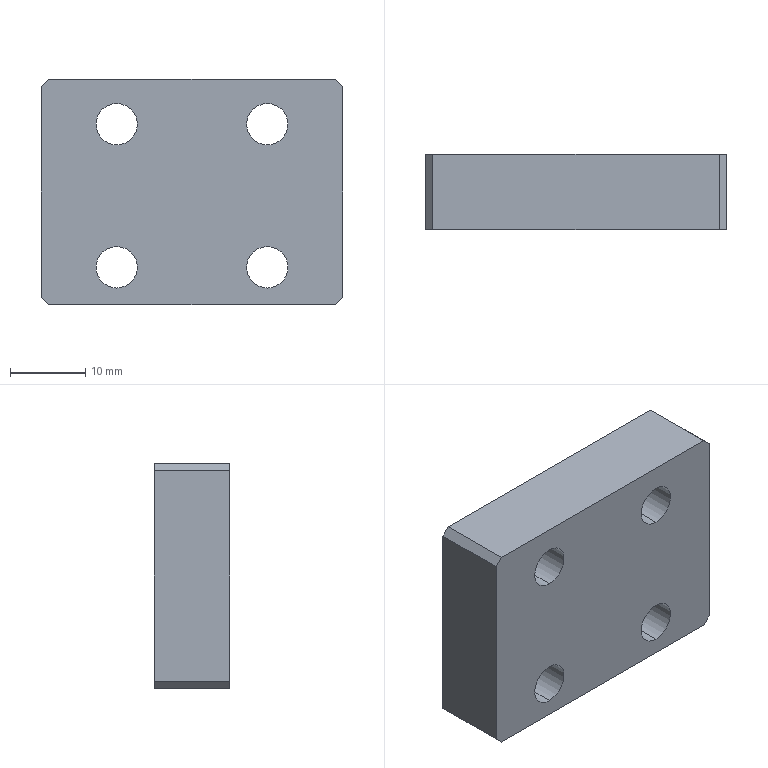Part | STEP file | 1 solid | 30 faces | box 40 x 10 x 30 mm | volume 9955 mm3 | cylinder 16 | plane 14 | commonest cylinder face diameters 5.5 x8 9.5 x8